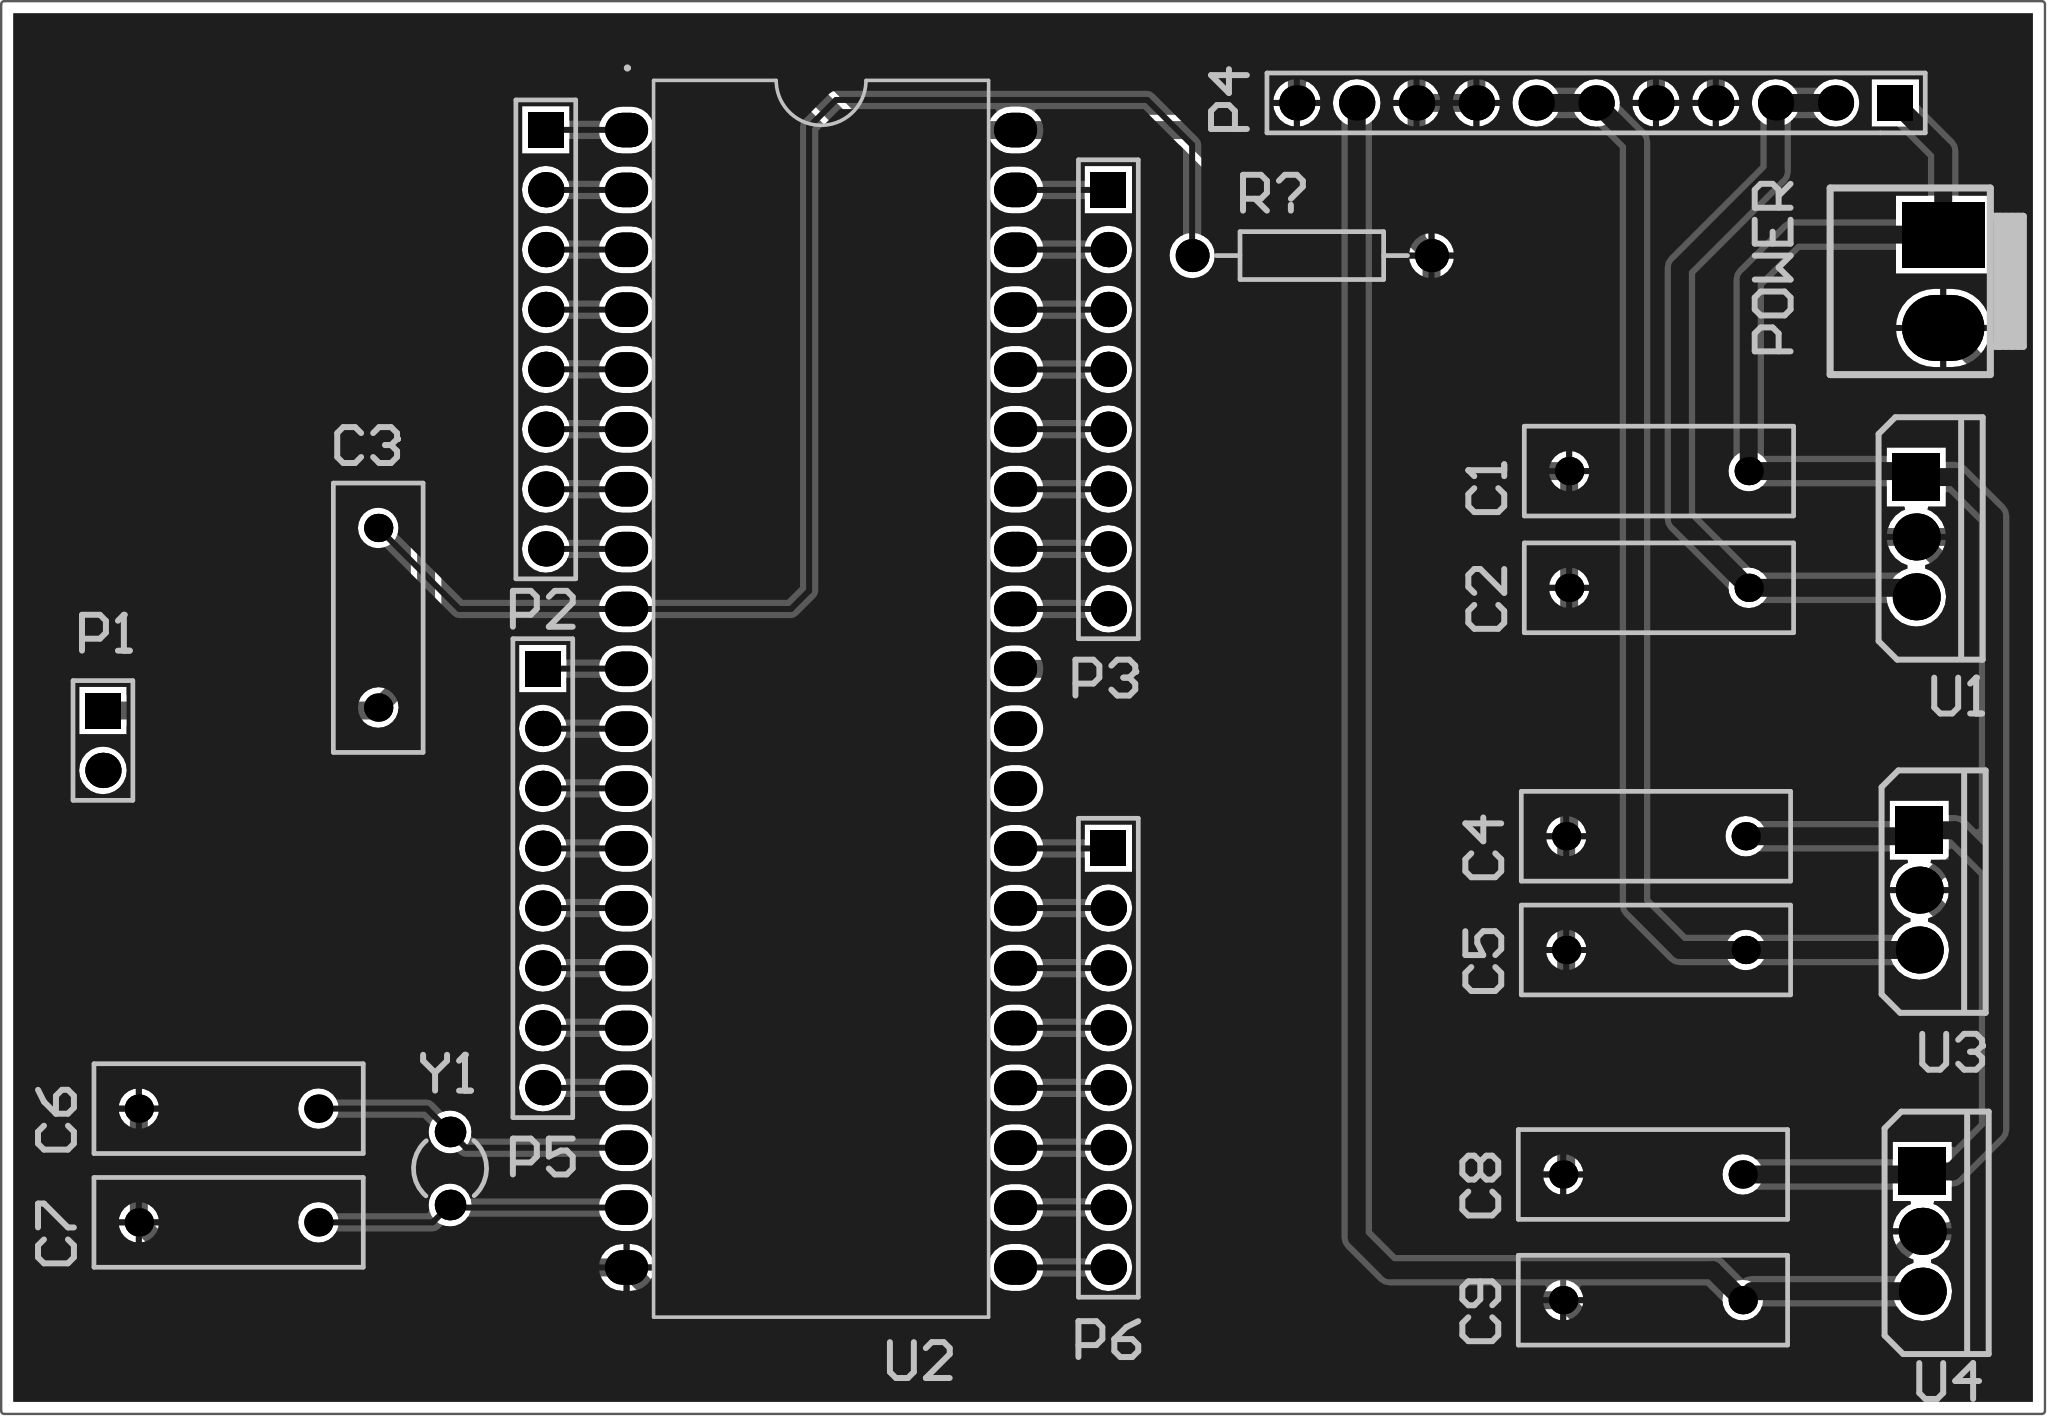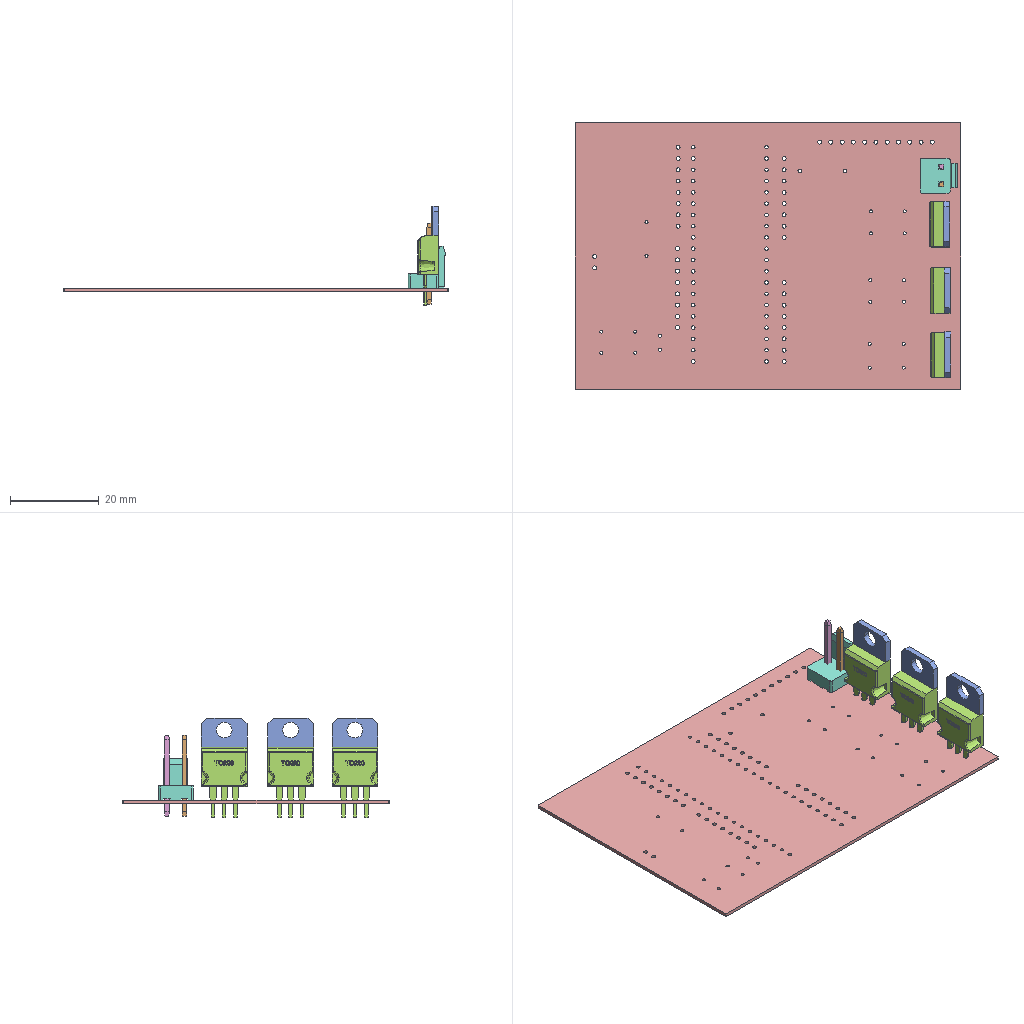Circuit board layout | Altium Designer | box 86.7 x 59.9 x 22.5 mm
Layer stack:
# Altium Designer layer stack of  (unit mm; dielectric type: 0 none, 1 core, 2 prepreg, 3 surface material)
index,name,kind,layer,copper_thickness_mm,dielectric_type,dielectric_thickness_mm,dielectric_material,dielectric_constant
0,Top Paste,other,,,,,,
1,Top Overlay,other,,,,,,
2,Top Solder,dielectric,,,3,0.0102,Solder Resist,3.5
3,Top Layer,copper,Top Layer,0.0356,,,,
4,Dielectric 1,dielectric,,,1,0.254,FR-4,4.2
5,GND,copper,GND,0.036,,,,
6,Dielectric 3,dielectric,,,2,0.127,,4.2
7,VCC,copper,VCC,0.036,,,,
8,Dielectric 2,dielectric,,,1,0.254,,4.2
9,Bottom Layer,copper,Bottom Layer,0.0356,,,,
10,Bottom Solder,dielectric,,,3,0.0102,Solder Resist,3.5
11,Bottom Overlay,other,,,,,,
12,Bottom Paste,other,,,,,,
# drill layer pairs: low layer,high layer
drill_pair,Top Layer,Bottom Layer
Part placement:
Designator,Comment,Layer,Footprint,Center-X(mm),Center-Y(mm),Rotation
Y1,XTAL,TopLayer,R38,77.851,42.037,180
U4,LM7806,TopLayer,TO220A,140.335,39.37,270
U3,LM7805,TopLayer,TO220A,140.208,53.848,270
U2,STC89C52RC,TopLayer,STC89C52RC,93.599,61.968,270
U1,LM7805,TopLayer,TO220A,140.081,68.834,270
R?,10K,TopLayer,AXIAL-0.4,114.427,80.772,180
POWER,Terminal block,TopLayer,VH3.96-2A,141.224,79.681,270
P6,Header 8,TopLayer,HDR1X8,105.791,46.736,270
P5,Header 8,TopLayer,HDR1X8,81.788,54.356,270
P4,Header 11,TopLayer,HDR1X11,126.492,87.249,180
P3,Header 8,TopLayer,HDR1X8,105.791,74.676,270
P2,Header 8,TopLayer,HDR1X8,81.915,77.216,270
P1,Header 2,TopLayer,HDR1X2,63.119,60.198,270
C9,0.1UF,TopLayer,RAD-0.3,128.905,36.449,180
C8,0.33UF,TopLayer,RAD-0.3,128.905,41.783,180
C7,22pF,TopLayer,RAD-0.3,68.453,39.751,180
C6,22pF,TopLayer,RAD-0.3,68.453,44.577,180
C5,0.1UF,TopLayer,RAD-0.3,129.032,51.308,180
C4,0.33UF,TopLayer,RAD-0.3,129.032,56.134,180
C3,10UF,TopLayer,RAD-0.3,74.803,65.405,90
C2,0.1UF,TopLayer,RAD-0.3,129.159,66.675,180
C1,0.33UF,TopLayer,RAD-0.3,129.159,71.628,180
Pad and via stacks:
# Altium Designer via and pad stacks of  (unit mm). Each distinct definition once, with the count of objects using it.
# via: kind,start_layer,end_layer,hole_mm,diameter_mm,mode(0 simple;1 top-mid-bottom;2 full stack),diameter_per_layer,count,example_net
# pad: kind,layer,hole_mm,hole_type(0 round;1 square;2 slot),plating,top_size,top_shape(1 round;2 rect;3 octagon;9 rounded rect),mid_size,bottom_size,mode,footprint,size_per_layer,count,example
pad,Multi-Layer,0.9,0,plated,1.5x1.5,1,1.5x1.5,1.5x1.5,0,HDR1X11,,10,P4.11
pad,Multi-Layer,0.9,0,plated,1.5x1.5,2,1.5x1.5,1.5x1.5,0,HDR1X11,,1,P4.1
pad,Multi-Layer,1.1,0,plated,2x2,1,2x2,2x2,0,TO220A,,6,U1.2
pad,Multi-Layer,1.1,0,plated,2x2,2,2x2,2x2,0,TO220A,,3,U1.1
pad,Multi-Layer,0.8,0,plated,1.467x1.833,1,1.467x1.833,1.467x1.833,0,STC89C52RC,,40,U2.1
pad,Multi-Layer,0.9,0,plated,1.5x1.5,2,1.5x1.5,1.5x1.5,0,HDR1X8,,4,P2.1
pad,Multi-Layer,0.9,0,plated,1.5x1.5,1,1.5x1.5,1.5x1.5,0,HDR1X8,,28,P2.2
pad,Multi-Layer,0.7,0,plated,1.2x1.2,1,1.2x1.2,1.2x1.2,0,RAD-0.3,,18,C2.2
pad,Multi-Layer,1.6,0,plated,2.8x3.5,2,2.8x3.5,2.8x3.5,0,VH3.96-2A,,1,POWER.1
pad,Multi-Layer,1.6,0,plated,2.8x3.5,1,2.8x3.5,2.8x3.5,0,VH3.96-2A,,1,POWER.2
pad,Multi-Layer,0.85,0,plated,1.4x1.4,1,1.4x1.4,1.4x1.4,0,AXIAL-0.4,,2,R?.1
pad,Multi-Layer,0.7,0,plated,1.3x1.3,1,1.3x1.3,1.3x1.3,0,R38,,2,Y1.1
pad,Multi-Layer,0.9,0,plated,1.5x1.5,2,1.5x1.5,1.5x1.5,0,HDR1X2,,1,P1.1
pad,Multi-Layer,0.9,0,plated,1.5x1.5,1,1.5x1.5,1.5x1.5,0,HDR1X2,,1,P1.2
Copper pours:
name,layer,net,type(0 solid;1 hatched;2 none)
D,Top Layer,GND,0
D,Bottom Layer,GND,0
Design rules, without the lines most boards share:
# Altium Designer design rules of  (exported by Altium Designer, unit mm)
# columns: name | kind | enabled | priority | scope1 | scope2 | descriptor | typed fields (field=value)
SilkToSilkClearance | 55 | enabled | 1 | All | All | Silk to Silk (Clearance=0mil) (All),(All) |
SilkToSolderMaskClearance | 54 | enabled | 1 | IsPad | All | Silk To Solder Mask (Clearance=0mil) (IsPad),(All) |
MinimumSolderMaskSliver | 53 | enabled | 1 | All | All | Minimum Solder Mask Sliver (Gap=0mil) (All),(All) |
HoleToHoleClearance | 52 | enabled | 1 | All | All | Hole To Hole Clearance (Gap=10mil) (All),(All) | gap=0.254
DiffPairsRouting | 51 | enabled | 1 | All | All | Differential Pairs Uncoupled Length using the Gap Constraints (Min=10mil) (Max=10mil) (Prefered=10mil)  and Width Constraints (Min=15mil) (Max=15mil) (Prefered=15mil) (All) |
SolderMaskExpansion | 13 | enabled | 1 | All | All | Solder Mask Expansion (Expansion =4mil) (All) | expansion=0.1016
RoutingVias | 11 | enabled | 1 | All | All | Routing Via (MinHoleWidth=28mil) (MaxHoleWidth=28mil) (PreferredHoleWidth=28mil) (MinWidth=50mil) (MaxWidth=50mil) (PreferedWidth=50mil) (All) | via_min_hole=0.7112 via_max_hole=0.7112 via_preferred_diameter=1.27 via_preferred_hole=0.7112
Width | 2 | enabled | 1 | All | All | Width Constraint (Min=10mil) (Max=50mil) (Preferred=10mil) (All) |
PolygonConnect | 20 | enabled | 1 | All | All | Polygon Connect Rule(Relief Connect )(Conductor Width=10mil) (Relief Angle=90 Angle) (Entries=4) (Air Gap Width=10mil) (All),(All) | connect_style(0=relief,1=direct,2=none)=0 relief_conductor_width=0.254 relief_entries=4
PlaneConnect | 6 | enabled | 1 | All | All | Power Plane Connect Rule(Relief Connect )(Expansion=20mil) (Conductor Width=10mil) (Air Gap=10mil) (Entries=4) (All) | relief_conductor_width=0.254 relief_entries=4 relief_expansion=0.508
Clearance | 0 | enabled | 1 | All | All | Clearance Constraint (Gap=10mil) (All),(All) | gap=0.254
Classes set for this board:
# Altium Designer classes of  (member kind: 0 net, 1 component, 2 from-to, 3 pad, 4 layer, 5 differential pair, 6 design channel, 7 polygon, 8 structure, 9 xSignal)
# columns: class name | member kind | superclass | members
Sheet2 | 1 | no | C1; C2; C3; C4; C5; C6; C7; C8; C9; P1; P2; P3; P4; P5; P6; POWER; R?; U1; U2; U3; U4; Y1;